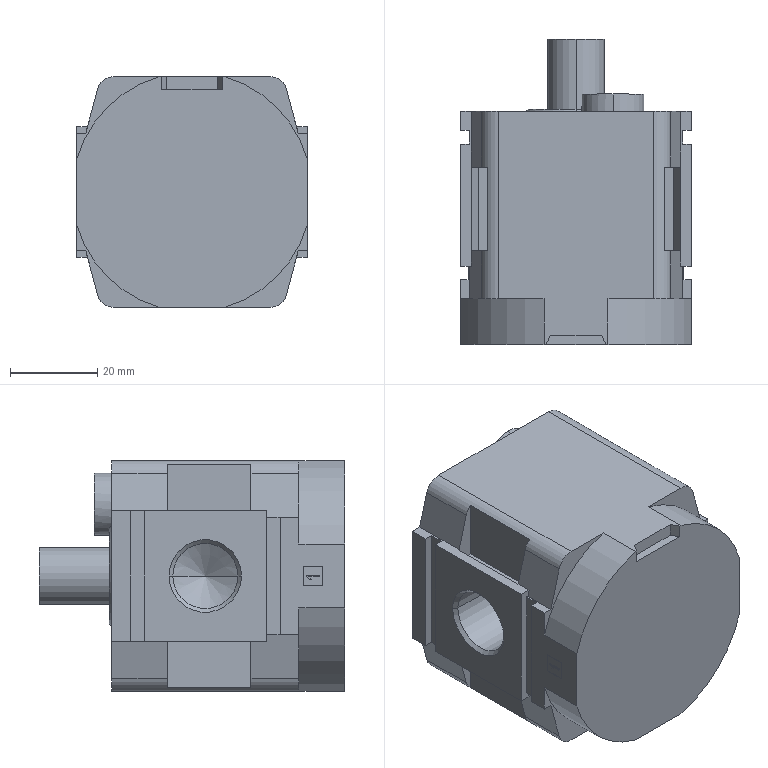Part | SolidWorks | features BaseBody 1 | 1 solid | 171 faces | box 53 x 70.1 x 53 mm | volume 131657 mm3 | plane 129 | cylinder 32 | cone 10 | commonest cylinder face diameters 8 x4 14.95 x4 55 x4 1.132 x2 1.336 x2 13.05 x2